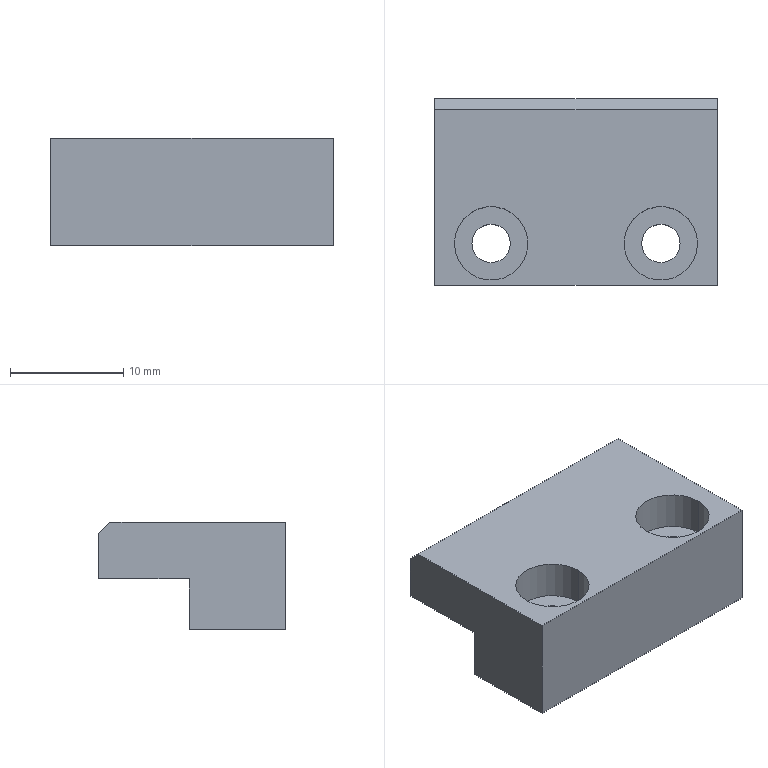Part | STEP file | PN_0054 | 1 solid | 19 faces | box 25 x 16.5 x 9.5 mm | volume 2670 mm3 | plane 11 | cylinder 8 | commonest cylinder face diameters 3.4 x4 6.5 x4
STEP:
#1=CARTESIAN_POINT('',(0.,0.,0.));
#2=DIRECTION('',(0.,0.,1.));
#3=DIRECTION('',(1.,0.,0.));
#4=AXIS2_PLACEMENT_3D('',#1,#2,#3);
#5=CARTESIAN_POINT('',(-4.25,-4.55,6.1));
#6=VERTEX_POINT('',#5);
#7=CARTESIAN_POINT('',(-4.25,-4.55,9.5));
#8=VERTEX_POINT('',#7);
#9=CARTESIAN_POINT('',(-4.25,-4.55,9.5));
#10=DIRECTION('',(0.,0.,1.));
#11=VECTOR('',#10,1.);
#12=LINE('',#9,#11);
#13=CARTESIAN_POINT('',(-7.5,-4.55,9.5));
#14=DIRECTION('',(0.,0.,1.));
#15=DIRECTION('',(1.,0.,0.));
#16=AXIS2_PLACEMENT_3D('',#13,#14,#15);
#17=CYLINDRICAL_SURFACE('',#16,3.25);
#18=CARTESIAN_POINT('',(6.283,0.));
#19=DIRECTION('',(0.,1.));
#20=VECTOR('',#19,1.);
#21=LINE('',#18,#20);
#22=(GEOMETRIC_REPRESENTATION_CONTEXT(2)PARAMETRIC_REPRESENTATION_CONTEXT()REPRESENTATION_CONTEXT('',''));
#23=DEFINITIONAL_REPRESENTATION('',(#21),#22);
#24=PCURVE('',#17,#23);
#25=CARTESIAN_POINT('',(-7.5,-4.55,9.5));
#26=DIRECTION('',(0.,0.,1.));
#27=DIRECTION('',(1.,0.,0.));
#28=AXIS2_PLACEMENT_3D('',#25,#26,#27);
#29=CYLINDRICAL_SURFACE('',#28,3.25);
#30=CARTESIAN_POINT('',(0.,0.));
#31=DIRECTION('',(0.,1.));
#32=VECTOR('',#31,1.);
#33=LINE('',#30,#32);
#34=(GEOMETRIC_REPRESENTATION_CONTEXT(2)PARAMETRIC_REPRESENTATION_CONTEXT()REPRESENTATION_CONTEXT('',''));
#35=DEFINITIONAL_REPRESENTATION('',(#33),#34);
#36=PCURVE('',#29,#35);
#37=SURFACE_CURVE('',#12,(#24,#36),.PCURVE_S1.);
#38=EDGE_CURVE('',#6,#8,#37,.T.);
#39=ORIENTED_EDGE('',*,*,#38,.T.);
#40=CARTESIAN_POINT('',(-10.75,-4.55,9.5));
#41=VERTEX_POINT('',#40);
#42=CARTESIAN_POINT('',(-7.5,-4.55,9.5));
#43=DIRECTION('',(0.,0.,1.));
#44=DIRECTION('',(1.,0.,0.));
#45=AXIS2_PLACEMENT_3D('',#42,#43,#44);
#46=CIRCLE('',#45,3.25);
#47=CARTESIAN_POINT('',(0.,0.));
#48=DIRECTION('',(1.,0.));
#49=VECTOR('',#48,1.);
#50=LINE('',#47,#49);
#51=(GEOMETRIC_REPRESENTATION_CONTEXT(2)PARAMETRIC_REPRESENTATION_CONTEXT()REPRESENTATION_CONTEXT('',''));
#52=DEFINITIONAL_REPRESENTATION('',(#50),#51);
#53=PCURVE('',#17,#52);
#54=CARTESIAN_POINT('',(0.,0.,9.5));
#55=DIRECTION('',(0.,0.,1.));
#56=DIRECTION('',(1.,0.,0.));
#57=AXIS2_PLACEMENT_3D('',#54,#55,#56);
#58=PLANE('',#57);
#59=CARTESIAN_POINT('',(-7.5,-4.55));
#60=DIRECTION('',(1.,0.));
#61=AXIS2_PLACEMENT_2D('',#59,#60);
#62=CIRCLE('',#61,3.25);
#63=(GEOMETRIC_REPRESENTATION_CONTEXT(2)PARAMETRIC_REPRESENTATION_CONTEXT()REPRESENTATION_CONTEXT('',''));
#64=DEFINITIONAL_REPRESENTATION('',(#62),#63);
#65=PCURVE('',#58,#64);
#66=SURFACE_CURVE('',#46,(#53,#65),.PCURVE_S1.);
#67=EDGE_CURVE('',#41,#8,#66,.T.);
#68=ORIENTED_EDGE('',*,*,#67,.F.);
#69=CARTESIAN_POINT('',(-10.75,-4.55,6.1));
#70=VERTEX_POINT('',#69);
#71=CARTESIAN_POINT('',(-10.75,-4.55,9.5));
#72=DIRECTION('',(0.,0.,1.));
#73=VECTOR('',#72,1.);
#74=LINE('',#71,#73);
#75=CARTESIAN_POINT('',(3.142,0.));
#76=DIRECTION('',(0.,1.));
#77=VECTOR('',#76,1.);
#78=LINE('',#75,#77);
#79=(GEOMETRIC_REPRESENTATION_CONTEXT(2)PARAMETRIC_REPRESENTATION_CONTEXT()REPRESENTATION_CONTEXT('',''));
#80=DEFINITIONAL_REPRESENTATION('',(#78),#79);
#81=PCURVE('',#17,#80);
#82=CARTESIAN_POINT('',(3.142,0.));
#83=DIRECTION('',(0.,1.));
#84=VECTOR('',#83,1.);
#85=LINE('',#82,#84);
#86=(GEOMETRIC_REPRESENTATION_CONTEXT(2)PARAMETRIC_REPRESENTATION_CONTEXT()REPRESENTATION_CONTEXT('',''));
#87=DEFINITIONAL_REPRESENTATION('',(#85),#86);
#88=PCURVE('',#29,#87);
#89=SURFACE_CURVE('',#74,(#81,#88),.PCURVE_S1.);
#90=EDGE_CURVE('',#70,#41,#89,.T.);
#91=ORIENTED_EDGE('',*,*,#90,.F.);
#92=CARTESIAN_POINT('',(-7.5,-4.55,6.1));
#93=DIRECTION('',(0.,0.,1.));
#94=DIRECTION('',(1.,0.,0.));
#95=AXIS2_PLACEMENT_3D('',#92,#93,#94);
#96=CIRCLE('',#95,3.25);
#97=CARTESIAN_POINT('',(0.,-3.4));
#98=DIRECTION('',(1.,0.));
#99=VECTOR('',#98,1.);
#100=LINE('',#97,#99);
#101=(GEOMETRIC_REPRESENTATION_CONTEXT(2)PARAMETRIC_REPRESENTATION_CONTEXT()REPRESENTATION_CONTEXT('',''));
#102=DEFINITIONAL_REPRESENTATION('',(#100),#101);
#103=PCURVE('',#17,#102);
#104=CARTESIAN_POINT('',(-5.8,-4.55,6.1));
#105=DIRECTION('',(0.,0.,-1.));
#106=DIRECTION('',(-1.,0.,0.));
#107=AXIS2_PLACEMENT_3D('',#104,#105,#106);
#108=PLANE('',#107);
#109=CARTESIAN_POINT('',(-1.55,0.));
#110=CARTESIAN_POINT('',(-1.55,5.629));
#111=CARTESIAN_POINT('',(3.325,2.815));
#112=CARTESIAN_POINT('',(8.2,0.));
#113=CARTESIAN_POINT('',(3.325,-2.815));
#114=CARTESIAN_POINT('',(-1.55,-5.629));
#115=CARTESIAN_POINT('',(-1.55,0.));
#116=(BOUNDED_CURVE()B_SPLINE_CURVE(2,(#109,#110,#111,#112,#113,#114,#115),.UNSPECIFIED.,.T.,.F.)B_SPLINE_CURVE_WITH_KNOTS((1,2,2,2,2,1),(-2.094,0.,2.094,4.189,6.283,8.378),.UNSPECIFIED.)CURVE()GEOMETRIC_REPRESENTATION_ITEM()RATIONAL_B_SPLINE_CURVE((1.,0.5,1.,0.5,1.,0.5,1.))REPRESENTATION_ITEM(''));
#117=(GEOMETRIC_REPRESENTATION_CONTEXT(2)PARAMETRIC_REPRESENTATION_CONTEXT()REPRESENTATION_CONTEXT('',''));
#118=DEFINITIONAL_REPRESENTATION('',(#116),#117);
#119=PCURVE('',#108,#118);
#120=SURFACE_CURVE('',#96,(#103,#119),.PCURVE_S1.);
#121=EDGE_CURVE('',#70,#6,#120,.T.);
#122=ORIENTED_EDGE('',*,*,#121,.T.);
#123=EDGE_LOOP('',(#39,#68,#91,#122));
#124=FACE_BOUND('',#123,.F.);
#125=ADVANCED_FACE('',(#124),#17,.F.);
#126=CARTESIAN_POINT('',(-5.8,-4.55,0.));
#127=VERTEX_POINT('',#126);
#128=CARTESIAN_POINT('',(-5.8,-4.55,6.1));
#129=VERTEX_POINT('',#128);
#130=CARTESIAN_POINT('',(-5.8,-4.55,9.5));
#131=DIRECTION('',(0.,0.,1.));
#132=VECTOR('',#131,1.);
#133=LINE('',#130,#132);
#134=CARTESIAN_POINT('',(-7.5,-4.55,9.5));
#135=DIRECTION('',(0.,0.,1.));
#136=DIRECTION('',(1.,0.,0.));
#137=AXIS2_PLACEMENT_3D('',#134,#135,#136);
#138=CYLINDRICAL_SURFACE('',#137,1.7);
#139=CARTESIAN_POINT('',(6.283,0.));
#140=DIRECTION('',(0.,1.));
#141=VECTOR('',#140,1.);
#142=LINE('',#139,#141);
#143=(GEOMETRIC_REPRESENTATION_CONTEXT(2)PARAMETRIC_REPRESENTATION_CONTEXT()REPRESENTATION_CONTEXT('',''));
#144=DEFINITIONAL_REPRESENTATION('',(#142),#143);
#145=PCURVE('',#138,#144);
#146=CARTESIAN_POINT('',(-7.5,-4.55,9.5));
#147=DIRECTION('',(0.,0.,1.));
#148=DIRECTION('',(1.,0.,0.));
#149=AXIS2_PLACEMENT_3D('',#146,#147,#148);
#150=CYLINDRICAL_SURFACE('',#149,1.7);
#151=CARTESIAN_POINT('',(0.,0.));
#152=DIRECTION('',(0.,1.));
#153=VECTOR('',#152,1.);
#154=LINE('',#151,#153);
#155=(GEOMETRIC_REPRESENTATION_CONTEXT(2)PARAMETRIC_REPRESENTATION_CONTEXT()REPRESENTATION_CONTEXT('',''));
#156=DEFINITIONAL_REPRESENTATION('',(#154),#155);
#157=PCURVE('',#150,#156);
#158=SURFACE_CURVE('',#133,(#145,#157),.PCURVE_S1.);
#159=EDGE_CURVE('',#127,#129,#158,.T.);
#160=ORIENTED_EDGE('',*,*,#159,.T.);
#161=CARTESIAN_POINT('',(-9.2,-4.55,6.1));
#162=VERTEX_POINT('',#161);
#163=CARTESIAN_POINT('',(-7.5,-4.55,6.1));
#164=DIRECTION('',(0.,0.,1.));
#165=DIRECTION('',(1.,0.,0.));
#166=AXIS2_PLACEMENT_3D('',#163,#164,#165);
#167=CIRCLE('',#166,1.7);
#168=CARTESIAN_POINT('',(0.,-3.4));
#169=DIRECTION('',(1.,0.));
#170=VECTOR('',#169,1.);
#171=LINE('',#168,#170);
#172=(GEOMETRIC_REPRESENTATION_CONTEXT(2)PARAMETRIC_REPRESENTATION_CONTEXT()REPRESENTATION_CONTEXT('',''));
#173=DEFINITIONAL_REPRESENTATION('',(#171),#172);
#174=PCURVE('',#138,#173);
#175=CARTESIAN_POINT('',(0.,0.));
#176=CARTESIAN_POINT('',(0.,2.944));
#177=CARTESIAN_POINT('',(2.55,1.472));
#178=CARTESIAN_POINT('',(5.1,0.));
#179=CARTESIAN_POINT('',(2.55,-1.472));
#180=CARTESIAN_POINT('',(0.,-2.944));
#181=CARTESIAN_POINT('',(0.,0.));
#182=(BOUNDED_CURVE()B_SPLINE_CURVE(2,(#175,#176,#177,#178,#179,#180,#181),.UNSPECIFIED.,.T.,.F.)B_SPLINE_CURVE_WITH_KNOTS((1,2,2,2,2,1),(-2.094,0.,2.094,4.189,6.283,8.378),.UNSPECIFIED.)CURVE()GEOMETRIC_REPRESENTATION_ITEM()RATIONAL_B_SPLINE_CURVE((1.,0.5,1.,0.5,1.,0.5,1.))REPRESENTATION_ITEM(''));
#183=(GEOMETRIC_REPRESENTATION_CONTEXT(2)PARAMETRIC_REPRESENTATION_CONTEXT()REPRESENTATION_CONTEXT('',''));
#184=DEFINITIONAL_REPRESENTATION('',(#182),#183);
#185=PCURVE('',#108,#184);
#186=SURFACE_CURVE('',#167,(#174,#185),.PCURVE_S1.);
#187=EDGE_CURVE('',#162,#129,#186,.T.);
#188=ORIENTED_EDGE('',*,*,#187,.F.);
#189=CARTESIAN_POINT('',(-9.2,-4.55,0.));
#190=VERTEX_POINT('',#189);
#191=CARTESIAN_POINT('',(-9.2,-4.55,9.5));
#192=DIRECTION('',(0.,0.,1.));
#193=VECTOR('',#192,1.);
#194=LINE('',#191,#193);
#195=CARTESIAN_POINT('',(3.142,0.));
#196=DIRECTION('',(0.,1.));
#197=VECTOR('',#196,1.);
#198=LINE('',#195,#197);
#199=(GEOMETRIC_REPRESENTATION_CONTEXT(2)PARAMETRIC_REPRESENTATION_CONTEXT()REPRESENTATION_CONTEXT('',''));
#200=DEFINITIONAL_REPRESENTATION('',(#198),#199);
#201=PCURVE('',#138,#200);
#202=CARTESIAN_POINT('',(3.142,0.));
#203=DIRECTION('',(0.,1.));
#204=VECTOR('',#203,1.);
#205=LINE('',#202,#204);
#206=(GEOMETRIC_REPRESENTATION_CONTEXT(2)PARAMETRIC_REPRESENTATION_CONTEXT()REPRESENTATION_CONTEXT('',''));
#207=DEFINITIONAL_REPRESENTATION('',(#205),#206);
#208=PCURVE('',#150,#207);
#209=SURFACE_CURVE('',#194,(#201,#208),.PCURVE_S1.);
#210=EDGE_CURVE('',#190,#162,#209,.T.);
#211=ORIENTED_EDGE('',*,*,#210,.F.);
#212=CARTESIAN_POINT('',(-7.5,-4.55,0.));
#213=DIRECTION('',(0.,0.,1.));
#214=DIRECTION('',(1.,0.,0.));
#215=AXIS2_PLACEMENT_3D('',#212,#213,#214);
#216=CIRCLE('',#215,1.7);
#217=CARTESIAN_POINT('',(0.,-9.5));
#218=DIRECTION('',(1.,0.));
#219=VECTOR('',#218,1.);
#220=LINE('',#217,#219);
#221=(GEOMETRIC_REPRESENTATION_CONTEXT(2)PARAMETRIC_REPRESENTATION_CONTEXT()REPRESENTATION_CONTEXT('',''));
#222=DEFINITIONAL_REPRESENTATION('',(#220),#221);
#223=PCURVE('',#138,#222);
#224=CARTESIAN_POINT('',(0.,0.,0.));
#225=DIRECTION('',(0.,0.,1.));
#226=DIRECTION('',(1.,0.,0.));
#227=AXIS2_PLACEMENT_3D('',#224,#225,#226);
#228=PLANE('',#227);
#229=CARTESIAN_POINT('',(-7.5,-4.55));
#230=DIRECTION('',(1.,0.));
#231=AXIS2_PLACEMENT_2D('',#229,#230);
#232=CIRCLE('',#231,1.7);
#233=(GEOMETRIC_REPRESENTATION_CONTEXT(2)PARAMETRIC_REPRESENTATION_CONTEXT()REPRESENTATION_CONTEXT('',''));
#234=DEFINITIONAL_REPRESENTATION('',(#232),#233);
#235=PCURVE('',#228,#234);
#236=SURFACE_CURVE('',#216,(#223,#235),.PCURVE_S1.);
#237=EDGE_CURVE('',#190,#127,#236,.T.);
#238=ORIENTED_EDGE('',*,*,#237,.T.);
#239=EDGE_LOOP('',(#160,#188,#211,#238));
#240=FACE_BOUND('',#239,.F.);
#241=ADVANCED_FACE('',(#240),#138,.F.);
#242=CARTESIAN_POINT('',(10.75,-4.55,6.1));
#243=VERTEX_POINT('',#242);
#244=CARTESIAN_POINT('',(10.75,-4.55,9.5));
#245=VERTEX_POINT('',#244);
#246=CARTESIAN_POINT('',(10.75,-4.55,9.5));
#247=DIRECTION('',(0.,0.,1.));
#248=VECTOR('',#247,1.);
#249=LINE('',#246,#248);
#250=CARTESIAN_POINT('',(7.5,-4.55,9.5));
#251=DIRECTION('',(0.,0.,1.));
#252=DIRECTION('',(1.,0.,0.));
#253=AXIS2_PLACEMENT_3D('',#250,#251,#252);
#254=CYLINDRICAL_SURFACE('',#253,3.25);
#255=CARTESIAN_POINT('',(6.283,0.));
#256=DIRECTION('',(0.,1.));
#257=VECTOR('',#256,1.);
#258=LINE('',#255,#257);
#259=(GEOMETRIC_REPRESENTATION_CONTEXT(2)PARAMETRIC_REPRESENTATION_CONTEXT()REPRESENTATION_CONTEXT('',''));
#260=DEFINITIONAL_REPRESENTATION('',(#258),#259);
#261=PCURVE('',#254,#260);
#262=CARTESIAN_POINT('',(7.5,-4.55,9.5));
#263=DIRECTION('',(0.,0.,1.));
#264=DIRECTION('',(1.,0.,0.));
#265=AXIS2_PLACEMENT_3D('',#262,#263,#264);
#266=CYLINDRICAL_SURFACE('',#265,3.25);
#267=CARTESIAN_POINT('',(0.,0.));
#268=DIRECTION('',(0.,1.));
#269=VECTOR('',#268,1.);
#270=LINE('',#267,#269);
#271=(GEOMETRIC_REPRESENTATION_CONTEXT(2)PARAMETRIC_REPRESENTATION_CONTEXT()REPRESENTATION_CONTEXT('',''));
#272=DEFINITIONAL_REPRESENTATION('',(#270),#271);
#273=PCURVE('',#266,#272);
#274=SURFACE_CURVE('',#249,(#261,#273),.PCURVE_S1.);
#275=EDGE_CURVE('',#243,#245,#274,.T.);
#276=ORIENTED_EDGE('',*,*,#275,.T.);
#277=CARTESIAN_POINT('',(4.25,-4.55,9.5));
#278=VERTEX_POINT('',#277);
#279=CARTESIAN_POINT('',(7.5,-4.55,9.5));
#280=DIRECTION('',(0.,0.,1.));
#281=DIRECTION('',(1.,0.,0.));
#282=AXIS2_PLACEMENT_3D('',#279,#280,#281);
#283=CIRCLE('',#282,3.25);
#284=CARTESIAN_POINT('',(0.,0.));
#285=DIRECTION('',(1.,0.));
#286=VECTOR('',#285,1.);
#287=LINE('',#284,#286);
#288=(GEOMETRIC_REPRESENTATION_CONTEXT(2)PARAMETRIC_REPRESENTATION_CONTEXT()REPRESENTATION_CONTEXT('',''));
#289=DEFINITIONAL_REPRESENTATION('',(#287),#288);
#290=PCURVE('',#254,#289);
#291=CARTESIAN_POINT('',(7.5,-4.55));
#292=DIRECTION('',(1.,0.));
#293=AXIS2_PLACEMENT_2D('',#291,#292);
#294=CIRCLE('',#293,3.25);
#295=(GEOMETRIC_REPRESENTATION_CONTEXT(2)PARAMETRIC_REPRESENTATION_CONTEXT()REPRESENTATION_CONTEXT('',''));
#296=DEFINITIONAL_REPRESENTATION('',(#294),#295);
#297=PCURVE('',#58,#296);
#298=SURFACE_CURVE('',#283,(#290,#297),.PCURVE_S1.);
#299=EDGE_CURVE('',#278,#245,#298,.T.);
#300=ORIENTED_EDGE('',*,*,#299,.F.);
#301=CARTESIAN_POINT('',(4.25,-4.55,6.1));
#302=VERTEX_POINT('',#301);
#303=CARTESIAN_POINT('',(4.25,-4.55,9.5));
#304=DIRECTION('',(0.,0.,1.));
#305=VECTOR('',#304,1.);
#306=LINE('',#303,#305);
#307=CARTESIAN_POINT('',(3.142,0.));
#308=DIRECTION('',(0.,1.));
#309=VECTOR('',#308,1.);
#310=LINE('',#307,#309);
#311=(GEOMETRIC_REPRESENTATION_CONTEXT(2)PARAMETRIC_REPRESENTATION_CONTEXT()REPRESENTATION_CONTEXT('',''));
#312=DEFINITIONAL_REPRESENTATION('',(#310),#311);
#313=PCURVE('',#254,#312);
#314=CARTESIAN_POINT('',(3.142,0.));
#315=DIRECTION('',(0.,1.));
#316=VECTOR('',#315,1.);
#317=LINE('',#314,#316);
#318=(GEOMETRIC_REPRESENTATION_CONTEXT(2)PARAMETRIC_REPRESENTATION_CONTEXT()REPRESENTATION_CONTEXT('',''));
#319=DEFINITIONAL_REPRESENTATION('',(#317),#318);
#320=PCURVE('',#266,#319);
#321=SURFACE_CURVE('',#306,(#313,#320),.PCURVE_S1.);
#322=EDGE_CURVE('',#302,#278,#321,.T.);
#323=ORIENTED_EDGE('',*,*,#322,.F.);
#324=CARTESIAN_POINT('',(7.5,-4.55,6.1));
#325=DIRECTION('',(0.,0.,1.));
#326=DIRECTION('',(1.,0.,0.));
#327=AXIS2_PLACEMENT_3D('',#324,#325,#326);
#328=CIRCLE('',#327,3.25);
#329=CARTESIAN_POINT('',(0.,-3.4));
#330=DIRECTION('',(1.,0.));
#331=VECTOR('',#330,1.);
#332=LINE('',#329,#331);
#333=(GEOMETRIC_REPRESENTATION_CONTEXT(2)PARAMETRIC_REPRESENTATION_CONTEXT()REPRESENTATION_CONTEXT('',''));
#334=DEFINITIONAL_REPRESENTATION('',(#332),#333);
#335=PCURVE('',#254,#334);
#336=CARTESIAN_POINT('',(9.2,-4.55,6.1));
#337=DIRECTION('',(0.,0.,-1.));
#338=DIRECTION('',(-1.,0.,0.));
#339=AXIS2_PLACEMENT_3D('',#336,#337,#338);
#340=PLANE('',#339);
#341=CARTESIAN_POINT('',(-1.55,0.));
#342=CARTESIAN_POINT('',(-1.55,5.629));
#343=CARTESIAN_POINT('',(3.325,2.815));
#344=CARTESIAN_POINT('',(8.2,0.));
#345=CARTESIAN_POINT('',(3.325,-2.815));
#346=CARTESIAN_POINT('',(-1.55,-5.629));
#347=CARTESIAN_POINT('',(-1.55,0.));
#348=(BOUNDED_CURVE()B_SPLINE_CURVE(2,(#341,#342,#343,#344,#345,#346,#347),.UNSPECIFIED.,.T.,.F.)B_SPLINE_CURVE_WITH_KNOTS((1,2,2,2,2,1),(-2.094,0.,2.094,4.189,6.283,8.378),.UNSPECIFIED.)CURVE()GEOMETRIC_REPRESENTATION_ITEM()RATIONAL_B_SPLINE_CURVE((1.,0.5,1.,0.5,1.,0.5,1.))REPRESENTATION_ITEM(''));
#349=(GEOMETRIC_REPRESENTATION_CONTEXT(2)PARAMETRIC_REPRESENTATION_CONTEXT()REPRESENTATION_CONTEXT('',''));
#350=DEFINITIONAL_REPRESENTATION('',(#348),#349);
#351=PCURVE('',#340,#350);
#352=SURFACE_CURVE('',#328,(#335,#351),.PCURVE_S1.);
#353=EDGE_CURVE('',#302,#243,#352,.T.);
#354=ORIENTED_EDGE('',*,*,#353,.T.);
#355=EDGE_LOOP('',(#276,#300,#323,#354));
#356=FACE_BOUND('',#355,.F.);
#357=ADVANCED_FACE('',(#356),#254,.F.);
#358=CARTESIAN_POINT('',(9.2,-4.55,0.));
#359=VERTEX_POINT('',#358);
#360=CARTESIAN_POINT('',(9.2,-4.55,6.1));
#361=VERTEX_POINT('',#360);
#362=CARTESIAN_POINT('',(9.2,-4.55,9.5));
#363=DIRECTION('',(0.,0.,1.));
#364=VECTOR('',#363,1.);
#365=LINE('',#362,#364);
#366=CARTESIAN_POINT('',(7.5,-4.55,9.5));
#367=DIRECTION('',(0.,0.,1.));
#368=DIRECTION('',(1.,0.,0.));
#369=AXIS2_PLACEMENT_3D('',#366,#367,#368);
#370=CYLINDRICAL_SURFACE('',#369,1.7);
#371=CARTESIAN_POINT('',(6.283,0.));
#372=DIRECTION('',(0.,1.));
#373=VECTOR('',#372,1.);
#374=LINE('',#371,#373);
#375=(GEOMETRIC_REPRESENTATION_CONTEXT(2)PARAMETRIC_REPRESENTATION_CONTEXT()REPRESENTATION_CONTEXT('',''));
#376=DEFINITIONAL_REPRESENTATION('',(#374),#375);
#377=PCURVE('',#370,#376);
#378=CARTESIAN_POINT('',(7.5,-4.55,9.5));
#379=DIRECTION('',(0.,0.,1.));
#380=DIRECTION('',(1.,0.,0.));
#381=AXIS2_PLACEMENT_3D('',#378,#379,#380);
#382=CYLINDRICAL_SURFACE('',#381,1.7);
#383=CARTESIAN_POINT('',(0.,0.));
#384=DIRECTION('',(0.,1.));
#385=VECTOR('',#384,1.);
#386=LINE('',#383,#385);
#387=(GEOMETRIC_REPRESENTATION_CONTEXT(2)PARAMETRIC_REPRESENTATION_CONTEXT()REPRESENTATION_CONTEXT('',''));
#388=DEFINITIONAL_REPRESENTATION('',(#386),#387);
#389=PCURVE('',#382,#388);
#390=SURFACE_CURVE('',#365,(#377,#389),.PCURVE_S1.);
#391=EDGE_CURVE('',#359,#361,#390,.T.);
#392=ORIENTED_EDGE('',*,*,#391,.T.);
#393=CARTESIAN_POINT('',(5.8,-4.55,6.1));
#394=VERTEX_POINT('',#393);
#395=CARTESIAN_POINT('',(7.5,-4.55,6.1));
#396=DIRECTION('',(0.,0.,1.));
#397=DIRECTION('',(1.,0.,0.));
#398=AXIS2_PLACEMENT_3D('',#395,#396,#397);
#399=CIRCLE('',#398,1.7);
#400=CARTESIAN_POINT('',(0.,-3.4));
#401=DIRECTION('',(1.,0.));
#402=VECTOR('',#401,1.);
#403=LINE('',#400,#402);
#404=(GEOMETRIC_REPRESENTATION_CONTEXT(2)PARAMETRIC_REPRESENTATION_CONTEXT()REPRESENTATION_CONTEXT('',''));
#405=DEFINITIONAL_REPRESENTATION('',(#403),#404);
#406=PCURVE('',#370,#405);
#407=CARTESIAN_POINT('',(0.,0.));
#408=CARTESIAN_POINT('',(0.,2.944));
#409=CARTESIAN_POINT('',(2.55,1.472));
#410=CARTESIAN_POINT('',(5.1,0.));
#411=CARTESIAN_POINT('',(2.55,-1.472));
#412=CARTESIAN_POINT('',(0.,-2.944));
#413=CARTESIAN_POINT('',(0.,0.));
#414=(BOUNDED_CURVE()B_SPLINE_CURVE(2,(#407,#408,#409,#410,#411,#412,#413),.UNSPECIFIED.,.T.,.F.)B_SPLINE_CURVE_WITH_KNOTS((1,2,2,2,2,1),(-2.094,0.,2.094,4.189,6.283,8.378),.UNSPECIFIED.)CURVE()GEOMETRIC_REPRESENTATION_ITEM()RATIONAL_B_SPLINE_CURVE((1.,0.5,1.,0.5,1.,0.5,1.))REPRESENTATION_ITEM(''));
#415=(GEOMETRIC_REPRESENTATION_CONTEXT(2)PARAMETRIC_REPRESENTATION_CONTEXT()REPRESENTATION_CONTEXT('',''));
#416=DEFINITIONAL_REPRESENTATION('',(#414),#415);
#417=PCURVE('',#340,#416);
#418=SURFACE_CURVE('',#399,(#406,#417),.PCURVE_S1.);
#419=EDGE_CURVE('',#394,#361,#418,.T.);
#420=ORIENTED_EDGE('',*,*,#419,.F.);
#421=CARTESIAN_POINT('',(5.8,-4.55,0.));
#422=VERTEX_POINT('',#421);
#423=CARTESIAN_POINT('',(5.8,-4.55,9.5));
#424=DIRECTION('',(0.,0.,1.));
#425=VECTOR('',#424,1.);
#426=LINE('',#423,#425);
#427=CARTESIAN_POINT('',(3.142,0.));
#428=DIRECTION('',(0.,1.));
#429=VECTOR('',#428,1.);
#430=LINE('',#427,#429);
#431=(GEOMETRIC_REPRESENTATION_CONTEXT(2)PARAMETRIC_REPRESENTATION_CONTEXT()REPRESENTATION_CONTEXT('',''));
#432=DEFINITIONAL_REPRESENTATION('',(#430),#431);
#433=PCURVE('',#370,#432);
#434=CARTESIAN_POINT('',(3.142,0.));
#435=DIRECTION('',(0.,1.));
#436=VECTOR('',#435,1.);
#437=LINE('',#434,#436);
#438=(GEOMETRIC_REPRESENTATION_CONTEXT(2)PARAMETRIC_REPRESENTATION_CONTEXT()REPRESENTATION_CONTEXT('',''));
#439=DEFINITIONAL_REPRESENTATION('',(#437),#438);
#440=PCURVE('',#382,#439);
#441=SURFACE_CURVE('',#426,(#433,#440),.PCURVE_S1.);
#442=EDGE_CURVE('',#422,#394,#441,.T.);
#443=ORIENTED_EDGE('',*,*,#442,.F.);
#444=CARTESIAN_POINT('',(7.5,-4.55,0.));
#445=DIRECTION('',(0.,0.,1.));
#446=DIRECTION('',(1.,0.,0.));
#447=AXIS2_PLACEMENT_3D('',#444,#445,#446);
#448=CIRCLE('',#447,1.7);
#449=CARTESIAN_POINT('',(0.,-9.5));
#450=DIRECTION('',(1.,0.));
#451=VECTOR('',#450,1.);
#452=LINE('',#449,#451);
#453=(GEOMETRIC_REPRESENTATION_CONTEXT(2)PARAMETRIC_REPRESENTATION_CONTEXT()REPRESENTATION_CONTEXT('',''));
#454=DEFINITIONAL_REPRESENTATION('',(#452),#453);
#455=PCURVE('',#370,#454);
#456=CARTESIAN_POINT('',(7.5,-4.55));
#457=DIRECTION('',(1.,0.));
#458=AXIS2_PLACEMENT_2D('',#456,#457);
#459=CIRCLE('',#458,1.7);
#460=(GEOMETRIC_REPRESENTATION_CONTEXT(2)PARAMETRIC_REPRESENTATION_CONTEXT()REPRESENTATION_CONTEXT('',''));
#461=DEFINITIONAL_REPRESENTATION('',(#459),#460);
#462=PCURVE('',#228,#461);
#463=SURFACE_CURVE('',#448,(#455,#462),.PCURVE_S1.);
#464=EDGE_CURVE('',#422,#359,#463,.T.);
#465=ORIENTED_EDGE('',*,*,#464,.T.);
#466=EDGE_LOOP('',(#392,#420,#443,#465));
#467=FACE_BOUND('',#466,.F.);
#468=ADVANCED_FACE('',(#467),#370,.F.);
#469=CARTESIAN_POINT('',(12.5,8.25,8.5));
#470=VERTEX_POINT('',#469);
#471=CARTESIAN_POINT('',(12.5,8.25,4.5));
#472=VERTEX_POINT('',#471);
#473=CARTESIAN_POINT('',(12.5,8.25,9.5));
#474=DIRECTION('',(0.,0.,-1.));
#475=VECTOR('',#474,1.);
#476=LINE('',#473,#475);
#477=CARTESIAN_POINT('',(12.5,8.25,9.5));
#478=DIRECTION('',(-1.,0.,0.));
#479=DIRECTION('',(0.,-1.,0.));
#480=AXIS2_PLACEMENT_3D('',#477,#478,#479);
#481=PLANE('',#480);
#482=CARTESIAN_POINT('',(0.,0.));
#483=DIRECTION('',(0.,-1.));
#484=VECTOR('',#483,1.);
#485=LINE('',#482,#484);
#486=(GEOMETRIC_REPRESENTATION_CONTEXT(2)PARAMETRIC_REPRESENTATION_CONTEXT()REPRESENTATION_CONTEXT('',''));
#487=DEFINITIONAL_REPRESENTATION('',(#485),#486);
#488=PCURVE('',#481,#487);
#489=CARTESIAN_POINT('',(-12.5,8.25,9.5));
#490=DIRECTION('',(0.,-1.,0.));
#491=DIRECTION('',(0.,0.,-1.));
#492=AXIS2_PLACEMENT_3D('',#489,#490,#491);
#493=PLANE('',#492);
#494=CARTESIAN_POINT('',(0.,25.));
#495=DIRECTION('',(1.,0.));
#496=VECTOR('',#495,1.);
#497=LINE('',#494,#496);
#498=(GEOMETRIC_REPRESENTATION_CONTEXT(2)PARAMETRIC_REPRESENTATION_CONTEXT()REPRESENTATION_CONTEXT('',''));
#499=DEFINITIONAL_REPRESENTATION('',(#497),#498);
#500=PCURVE('',#493,#499);
#501=SURFACE_CURVE('',#476,(#488,#500),.PCURVE_S1.);
#502=EDGE_CURVE('',#470,#472,#501,.T.);
#503=ORIENTED_EDGE('',*,*,#502,.F.);
#504=CARTESIAN_POINT('',(12.5,7.25,9.5));
#505=VERTEX_POINT('',#504);
#506=CARTESIAN_POINT('',(12.5,7.25,9.5));
#507=DIRECTION('',(0.,-0.7071,0.7071));
#508=VECTOR('',#507,1.);
#509=LINE('',#506,#508);
#510=CARTESIAN_POINT('',(1.,0.));
#511=DIRECTION('',(0.7071,0.7071));
#512=VECTOR('',#511,1.);
#513=LINE('',#510,#512);
#514=(GEOMETRIC_REPRESENTATION_CONTEXT(2)PARAMETRIC_REPRESENTATION_CONTEXT()REPRESENTATION_CONTEXT('',''));
#515=DEFINITIONAL_REPRESENTATION('',(#513),#514);
#516=PCURVE('',#481,#515);
#517=CARTESIAN_POINT('',(0.,7.25,9.5));
#518=DIRECTION('',(0.,0.7071,0.7071));
#519=DIRECTION('',(1.,0.,0.));
#520=AXIS2_PLACEMENT_3D('',#517,#518,#519);
#521=PLANE('',#520);
#522=CARTESIAN_POINT('',(12.5,0.));
#523=DIRECTION('',(0.,-1.));
#524=VECTOR('',#523,1.);
#525=LINE('',#522,#524);
#526=(GEOMETRIC_REPRESENTATION_CONTEXT(2)PARAMETRIC_REPRESENTATION_CONTEXT()REPRESENTATION_CONTEXT('',''));
#527=DEFINITIONAL_REPRESENTATION('',(#525),#526);
#528=PCURVE('',#521,#527);
#529=SURFACE_CURVE('',#509,(#516,#528),.PCURVE_S1.);
#530=EDGE_CURVE('',#470,#505,#529,.T.);
#531=ORIENTED_EDGE('',*,*,#530,.T.);
#532=CARTESIAN_POINT('',(12.5,-8.25,9.5));
#533=VERTEX_POINT('',#532);
#534=CARTESIAN_POINT('',(12.5,8.25,9.5));
#535=DIRECTION('',(0.,1.,0.));
#536=VECTOR('',#535,1.);
#537=LINE('',#534,#536);
#538=CARTESIAN_POINT('',(0.,0.));
#539=DIRECTION('',(-1.,0.));
#540=VECTOR('',#539,1.);
#541=LINE('',#538,#540);
#542=(GEOMETRIC_REPRESENTATION_CONTEXT(2)PARAMETRIC_REPRESENTATION_CONTEXT()REPRESENTATION_CONTEXT('',''));
#543=DEFINITIONAL_REPRESENTATION('',(#541),#542);
#544=PCURVE('',#481,#543);
#545=CARTESIAN_POINT('',(12.5,8.25));
#546=DIRECTION('',(0.,1.));
#547=VECTOR('',#546,1.);
#548=LINE('',#545,#547);
#549=(GEOMETRIC_REPRESENTATION_CONTEXT(2)PARAMETRIC_REPRESENTATION_CONTEXT()REPRESENTATION_CONTEXT('',''));
#550=DEFINITIONAL_REPRESENTATION('',(#548),#549);
#551=PCURVE('',#58,#550);
#552=SURFACE_CURVE('',#537,(#544,#551),.PCURVE_S1.);
#553=EDGE_CURVE('',#533,#505,#552,.T.);
#554=ORIENTED_EDGE('',*,*,#553,.F.);
#555=CARTESIAN_POINT('',(12.5,-8.25,0.));
#556=VERTEX_POINT('',#555);
#557=CARTESIAN_POINT('',(12.5,-8.25,9.5));
#558=DIRECTION('',(0.,0.,-1.));
#559=VECTOR('',#558,1.);
#560=LINE('',#557,#559);
#561=CARTESIAN_POINT('',(16.5,0.));
#562=DIRECTION('',(0.,-1.));
#563=VECTOR('',#562,1.);
#564=LINE('',#561,#563);
#565=(GEOMETRIC_REPRESENTATION_CONTEXT(2)PARAMETRIC_REPRESENTATION_CONTEXT()REPRESENTATION_CONTEXT('',''));
#566=DEFINITIONAL_REPRESENTATION('',(#564),#565);
#567=PCURVE('',#481,#566);
#568=CARTESIAN_POINT('',(-12.5,-8.25,9.5));
#569=DIRECTION('',(0.,1.,0.));
#570=DIRECTION('',(0.,0.,1.));
#571=AXIS2_PLACEMENT_3D('',#568,#569,#570);
#572=PLANE('',#571);
#573=CARTESIAN_POINT('',(0.,25.));
#574=DIRECTION('',(-1.,0.));
#575=VECTOR('',#574,1.);
#576=LINE('',#573,#575);
#577=(GEOMETRIC_REPRESENTATION_CONTEXT(2)PARAMETRIC_REPRESENTATION_CONTEXT()REPRESENTATION_CONTEXT('',''));
#578=DEFINITIONAL_REPRESENTATION('',(#576),#577);
#579=PCURVE('',#572,#578);
#580=SURFACE_CURVE('',#560,(#567,#579),.PCURVE_S1.);
#581=EDGE_CURVE('',#533,#556,#580,.T.);
#582=ORIENTED_EDGE('',*,*,#581,.T.);
#583=CARTESIAN_POINT('',(12.5,0.25,0.));
#584=VERTEX_POINT('',#583);
#585=CARTESIAN_POINT('',(12.5,8.25,0.));
#586=DIRECTION('',(0.,1.,0.));
#587=VECTOR('',#586,1.);
#588=LINE('',#585,#587);
#589=CARTESIAN_POINT('',(0.,-9.5));
#590=DIRECTION('',(-1.,0.));
#591=VECTOR('',#590,1.);
#592=LINE('',#589,#591);
#593=(GEOMETRIC_REPRESENTATION_CONTEXT(2)PARAMETRIC_REPRESENTATION_CONTEXT()REPRESENTATION_CONTEXT('',''));
#594=DEFINITIONAL_REPRESENTATION('',(#592),#593);
#595=PCURVE('',#481,#594);
#596=CARTESIAN_POINT('',(12.5,8.25));
#597=DIRECTION('',(0.,1.));
#598=VECTOR('',#597,1.);
#599=LINE('',#596,#598);
#600=(GEOMETRIC_REPRESENTATION_CONTEXT(2)PARAMETRIC_REPRESENTATION_CONTEXT()REPRESENTATION_CONTEXT('',''));
#601=DEFINITIONAL_REPRESENTATION('',(#599),#600);
#602=PCURVE('',#228,#601);
#603=SURFACE_CURVE('',#588,(#595,#602),.PCURVE_S1.);
#604=EDGE_CURVE('',#556,#584,#603,.T.);
#605=ORIENTED_EDGE('',*,*,#604,.T.);
#606=CARTESIAN_POINT('',(12.5,0.25,4.5));
#607=VERTEX_POINT('',#606);
#608=CARTESIAN_POINT('',(12.5,0.25,4.5));
#609=DIRECTION('',(0.,0.,-1.));
#610=VECTOR('',#609,1.);
#611=LINE('',#608,#610);
#612=CARTESIAN_POINT('',(8.,-5.));
#613=DIRECTION('',(0.,-1.));
#614=VECTOR('',#613,1.);
#615=LINE('',#612,#614);
#616=(GEOMETRIC_REPRESENTATION_CONTEXT(2)PARAMETRIC_REPRESENTATION_CONTEXT()REPRESENTATION_CONTEXT('',''));
#617=DEFINITIONAL_REPRESENTATION('',(#615),#616);
#618=PCURVE('',#481,#617);
#619=CARTESIAN_POINT('',(-12.5,0.25,4.5));
#620=DIRECTION('',(0.,-1.,0.));
#621=DIRECTION('',(1.,0.,0.));
#622=AXIS2_PLACEMENT_3D('',#619,#620,#621);
#623=PLANE('',#622);
#624=CARTESIAN_POINT('',(25.,0.));
#625=DIRECTION('',(0.,-1.));
#626=VECTOR('',#625,1.);
#627=LINE('',#624,#626);
#628=(GEOMETRIC_REPRESENTATION_CONTEXT(2)PARAMETRIC_REPRESENTATION_CONTEXT()REPRESENTATION_CONTEXT('',''));
#629=DEFINITIONAL_REPRESENTATION('',(#627),#628);
#630=PCURVE('',#623,#629);
#631=SURFACE_CURVE('',#611,(#618,#630),.PCURVE_S1.);
#632=EDGE_CURVE('',#607,#584,#631,.T.);
#633=ORIENTED_EDGE('',*,*,#632,.F.);
#634=CARTESIAN_POINT('',(12.5,8.25,4.5));
#635=DIRECTION('',(0.,-1.,0.));
#636=VECTOR('',#635,1.);
#637=LINE('',#634,#636);
#638=CARTESIAN_POINT('',(0.,-5.));
#639=DIRECTION('',(1.,0.));
#640=VECTOR('',#639,1.);
#641=LINE('',#638,#640);
#642=(GEOMETRIC_REPRESENTATION_CONTEXT(2)PARAMETRIC_REPRESENTATION_CONTEXT()REPRESENTATION_CONTEXT('',''));
#643=DEFINITIONAL_REPRESENTATION('',(#641),#642);
#644=PCURVE('',#481,#643);
#645=CARTESIAN_POINT('',(-12.5,8.25,4.5));
#646=DIRECTION('',(0.,0.,1.));
#647=DIRECTION('',(1.,0.,0.));
#648=AXIS2_PLACEMENT_3D('',#645,#646,#647);
#649=PLANE('',#648);
#650=CARTESIAN_POINT('',(25.,0.));
#651=DIRECTION('',(0.,-1.));
#652=VECTOR('',#651,1.);
#653=LINE('',#650,#652);
#654=(GEOMETRIC_REPRESENTATION_CONTEXT(2)PARAMETRIC_REPRESENTATION_CONTEXT()REPRESENTATION_CONTEXT('',''));
#655=DEFINITIONAL_REPRESENTATION('',(#653),#654);
#656=PCURVE('',#649,#655);
#657=SURFACE_CURVE('',#637,(#644,#656),.PCURVE_S1.);
#658=EDGE_CURVE('',#472,#607,#657,.T.);
#659=ORIENTED_EDGE('',*,*,#658,.F.);
#660=EDGE_LOOP('',(#503,#531,#554,#582,#605,#633,#659));
#661=FACE_BOUND('',#660,.T.);
#662=ADVANCED_FACE('',(#661),#481,.F.);
#663=CARTESIAN_POINT('',(-12.5,8.25,8.5));
#664=VERTEX_POINT('',#663);
#665=CARTESIAN_POINT('',(-12.5,8.25,4.5));
#666=VERTEX_POINT('',#665);
#667=CARTESIAN_POINT('',(-12.5,8.25,9.5));
#668=DIRECTION('',(0.,0.,-1.));
#669=VECTOR('',#668,1.);
#670=LINE('',#667,#669);
#671=CARTESIAN_POINT('',(0.,0.));
#672=DIRECTION('',(1.,0.));
#673=VECTOR('',#672,1.);
#674=LINE('',#671,#673);
#675=(GEOMETRIC_REPRESENTATION_CONTEXT(2)PARAMETRIC_REPRESENTATION_CONTEXT()REPRESENTATION_CONTEXT('',''));
#676=DEFINITIONAL_REPRESENTATION('',(#674),#675);
#677=PCURVE('',#493,#676);
#678=CARTESIAN_POINT('',(-12.5,8.25,9.5));
#679=DIRECTION('',(1.,0.,0.));
#680=DIRECTION('',(0.,1.,0.));
#681=AXIS2_PLACEMENT_3D('',#678,#679,#680);
#682=PLANE('',#681);
#683=CARTESIAN_POINT('',(0.,0.));
#684=DIRECTION('',(0.,-1.));
#685=VECTOR('',#684,1.);
#686=LINE('',#683,#685);
#687=(GEOMETRIC_REPRESENTATION_CONTEXT(2)PARAMETRIC_REPRESENTATION_CONTEXT()REPRESENTATION_CONTEXT('',''));
#688=DEFINITIONAL_REPRESENTATION('',(#686),#687);
#689=PCURVE('',#682,#688);
#690=SURFACE_CURVE('',#670,(#677,#689),.PCURVE_S1.);
#691=EDGE_CURVE('',#664,#666,#690,.T.);
#692=ORIENTED_EDGE('',*,*,#691,.F.);
#693=CARTESIAN_POINT('',(12.5,8.25,8.5));
#694=DIRECTION('',(1.,0.,0.));
#695=VECTOR('',#694,1.);
#696=LINE('',#693,#695);
#697=CARTESIAN_POINT('',(1.,25.));
#698=DIRECTION('',(0.,1.));
#699=VECTOR('',#698,1.);
#700=LINE('',#697,#699);
#701=(GEOMETRIC_REPRESENTATION_CONTEXT(2)PARAMETRIC_REPRESENTATION_CONTEXT()REPRESENTATION_CONTEXT('',''));
#702=DEFINITIONAL_REPRESENTATION('',(#700),#701);
#703=PCURVE('',#493,#702);
#704=CARTESIAN_POINT('',(12.5,1.414));
#705=DIRECTION('',(1.,0.));
#706=VECTOR('',#705,1.);
#707=LINE('',#704,#706);
#708=(GEOMETRIC_REPRESENTATION_CONTEXT(2)PARAMETRIC_REPRESENTATION_CONTEXT()REPRESENTATION_CONTEXT('',''));
#709=DEFINITIONAL_REPRESENTATION('',(#707),#708);
#710=PCURVE('',#521,#709);
#711=SURFACE_CURVE('',#696,(#703,#710),.PCURVE_S1.);
#712=EDGE_CURVE('',#664,#470,#711,.T.);
#713=ORIENTED_EDGE('',*,*,#712,.T.);
#714=ORIENTED_EDGE('',*,*,#502,.T.);
#715=CARTESIAN_POINT('',(-12.5,8.25,4.5));
#716=DIRECTION('',(1.,0.,0.));
#717=VECTOR('',#716,1.);
#718=LINE('',#715,#717);
#719=CARTESIAN_POINT('',(5.,0.));
#720=DIRECTION('',(0.,1.));
#721=VECTOR('',#720,1.);
#722=LINE('',#719,#721);
#723=(GEOMETRIC_REPRESENTATION_CONTEXT(2)PARAMETRIC_REPRESENTATION_CONTEXT()REPRESENTATION_CONTEXT('',''));
#724=DEFINITIONAL_REPRESENTATION('',(#722),#723);
#725=PCURVE('',#493,#724);
#726=CARTESIAN_POINT('',(0.,0.));
#727=DIRECTION('',(1.,0.));
#728=VECTOR('',#727,1.);
#729=LINE('',#726,#728);
#730=(GEOMETRIC_REPRESENTATION_CONTEXT(2)PARAMETRIC_REPRESENTATION_CONTEXT()REPRESENTATION_CONTEXT('',''));
#731=DEFINITIONAL_REPRESENTATION('',(#729),#730);
#732=PCURVE('',#649,#731);
#733=SURFACE_CURVE('',#718,(#725,#732),.PCURVE_S1.);
#734=EDGE_CURVE('',#666,#472,#733,.T.);
#735=ORIENTED_EDGE('',*,*,#734,.F.);
#736=EDGE_LOOP('',(#692,#713,#714,#735));
#737=FACE_BOUND('',#736,.T.);
#738=ADVANCED_FACE('',(#737),#493,.F.);
#739=CARTESIAN_POINT('',(-12.5,7.25,9.5));
#740=VERTEX_POINT('',#739);
#741=CARTESIAN_POINT('',(-12.5,-8.25,9.5));
#742=VERTEX_POINT('',#741);
#743=CARTESIAN_POINT('',(-12.5,8.25,9.5));
#744=DIRECTION('',(0.,-1.,0.));
#745=VECTOR('',#744,1.);
#746=LINE('',#743,#745);
#747=CARTESIAN_POINT('',(0.,0.));
#748=DIRECTION('',(-1.,0.));
#749=VECTOR('',#748,1.);
#750=LINE('',#747,#749);
#751=(GEOMETRIC_REPRESENTATION_CONTEXT(2)PARAMETRIC_REPRESENTATION_CONTEXT()REPRESENTATION_CONTEXT('',''));
#752=DEFINITIONAL_REPRESENTATION('',(#750),#751);
#753=PCURVE('',#682,#752);
#754=CARTESIAN_POINT('',(-12.5,8.25));
#755=DIRECTION('',(0.,-1.));
#756=VECTOR('',#755,1.);
#757=LINE('',#754,#756);
#758=(GEOMETRIC_REPRESENTATION_CONTEXT(2)PARAMETRIC_REPRESENTATION_CONTEXT()REPRESENTATION_CONTEXT('',''));
#759=DEFINITIONAL_REPRESENTATION('',(#757),#758);
#760=PCURVE('',#58,#759);
#761=SURFACE_CURVE('',#746,(#753,#760),.PCURVE_S1.);
#762=EDGE_CURVE('',#740,#742,#761,.T.);
#763=ORIENTED_EDGE('',*,*,#762,.F.);
#764=CARTESIAN_POINT('',(-12.5,7.25,9.5));
#765=DIRECTION('',(0.,0.7071,-0.7071));
#766=VECTOR('',#765,1.);
#767=LINE('',#764,#766);
#768=CARTESIAN_POINT('',(-1.,0.));
#769=DIRECTION('',(0.7071,-0.7071));
#770=VECTOR('',#769,1.);
#771=LINE('',#768,#770);
#772=(GEOMETRIC_REPRESENTATION_CONTEXT(2)PARAMETRIC_REPRESENTATION_CONTEXT()REPRESENTATION_CONTEXT('',''));
#773=DEFINITIONAL_REPRESENTATION('',(#771),#772);
#774=PCURVE('',#682,#773);
#775=CARTESIAN_POINT('',(-12.5,0.));
#776=DIRECTION('',(0.,1.));
#777=VECTOR('',#776,1.);
#778=LINE('',#775,#777);
#779=(GEOMETRIC_REPRESENTATION_CONTEXT(2)PARAMETRIC_REPRESENTATION_CONTEXT()REPRESENTATION_CONTEXT('',''));
#780=DEFINITIONAL_REPRESENTATION('',(#778),#779);
#781=PCURVE('',#521,#780);
#782=SURFACE_CURVE('',#767,(#774,#781),.PCURVE_S1.);
#783=EDGE_CURVE('',#740,#664,#782,.T.);
#784=ORIENTED_EDGE('',*,*,#783,.T.);
#785=ORIENTED_EDGE('',*,*,#691,.T.);
#786=CARTESIAN_POINT('',(-12.5,0.25,4.5));
#787=VERTEX_POINT('',#786);
#788=CARTESIAN_POINT('',(-12.5,8.25,4.5));
#789=DIRECTION('',(0.,-1.,0.));
#790=VECTOR('',#789,1.);
#791=LINE('',#788,#790);
#792=CARTESIAN_POINT('',(0.,-5.));
#793=DIRECTION('',(-1.,0.));
#794=VECTOR('',#793,1.);
#795=LINE('',#792,#794);
#796=(GEOMETRIC_REPRESENTATION_CONTEXT(2)PARAMETRIC_REPRESENTATION_CONTEXT()REPRESENTATION_CONTEXT('',''));
#797=DEFINITIONAL_REPRESENTATION('',(#795),#796);
#798=PCURVE('',#682,#797);
#799=CARTESIAN_POINT('',(0.,0.));
#800=DIRECTION('',(0.,-1.));
#801=VECTOR('',#800,1.);
#802=LINE('',#799,#801);
#803=(GEOMETRIC_REPRESENTATION_CONTEXT(2)PARAMETRIC_REPRESENTATION_CONTEXT()REPRESENTATION_CONTEXT('',''));
#804=DEFINITIONAL_REPRESENTATION('',(#802),#803);
#805=PCURVE('',#649,#804);
#806=SURFACE_CURVE('',#791,(#798,#805),.PCURVE_S1.);
#807=EDGE_CURVE('',#666,#787,#806,.T.);
#808=ORIENTED_EDGE('',*,*,#807,.T.);
#809=CARTESIAN_POINT('',(-12.5,0.25,0.));
#810=VERTEX_POINT('',#809);
#811=CARTESIAN_POINT('',(-12.5,0.25,4.5));
#812=DIRECTION('',(0.,0.,-1.));
#813=VECTOR('',#812,1.);
#814=LINE('',#811,#813);
#815=CARTESIAN_POINT('',(-8.,-5.));
#816=DIRECTION('',(0.,-1.));
#817=VECTOR('',#816,1.);
#818=LINE('',#815,#817);
#819=(GEOMETRIC_REPRESENTATION_CONTEXT(2)PARAMETRIC_REPRESENTATION_CONTEXT()REPRESENTATION_CONTEXT('',''));
#820=DEFINITIONAL_REPRESENTATION('',(#818),#819);
#821=PCURVE('',#682,#820);
#822=CARTESIAN_POINT('',(0.,0.));
#823=DIRECTION('',(0.,-1.));
#824=VECTOR('',#823,1.);
#825=LINE('',#822,#824);
#826=(GEOMETRIC_REPRESENTATION_CONTEXT(2)PARAMETRIC_REPRESENTATION_CONTEXT()REPRESENTATION_CONTEXT('',''));
#827=DEFINITIONAL_REPRESENTATION('',(#825),#826);
#828=PCURVE('',#623,#827);
#829=SURFACE_CURVE('',#814,(#821,#828),.PCURVE_S1.);
#830=EDGE_CURVE('',#787,#810,#829,.T.);
#831=ORIENTED_EDGE('',*,*,#830,.T.);
#832=CARTESIAN_POINT('',(-12.5,-8.25,0.));
#833=VERTEX_POINT('',#832);
#834=CARTESIAN_POINT('',(-12.5,8.25,0.));
#835=DIRECTION('',(0.,-1.,0.));
#836=VECTOR('',#835,1.);
#837=LINE('',#834,#836);
#838=CARTESIAN_POINT('',(0.,-9.5));
#839=DIRECTION('',(-1.,0.));
#840=VECTOR('',#839,1.);
#841=LINE('',#838,#840);
#842=(GEOMETRIC_REPRESENTATION_CONTEXT(2)PARAMETRIC_REPRESENTATION_CONTEXT()REPRESENTATION_CONTEXT('',''));
#843=DEFINITIONAL_REPRESENTATION('',(#841),#842);
#844=PCURVE('',#682,#843);
#845=CARTESIAN_POINT('',(-12.5,8.25));
#846=DIRECTION('',(0.,-1.));
#847=VECTOR('',#846,1.);
#848=LINE('',#845,#847);
#849=(GEOMETRIC_REPRESENTATION_CONTEXT(2)PARAMETRIC_REPRESENTATION_CONTEXT()REPRESENTATION_CONTEXT('',''));
#850=DEFINITIONAL_REPRESENTATION('',(#848),#849);
#851=PCURVE('',#228,#850);
#852=SURFACE_CURVE('',#837,(#844,#851),.PCURVE_S1.);
#853=EDGE_CURVE('',#810,#833,#852,.T.);
#854=ORIENTED_EDGE('',*,*,#853,.T.);
#855=CARTESIAN_POINT('',(-12.5,-8.25,9.5));
#856=DIRECTION('',(0.,0.,-1.));
#857=VECTOR('',#856,1.);
#858=LINE('',#855,#857);
#859=CARTESIAN_POINT('',(-16.5,0.));
#860=DIRECTION('',(0.,-1.));
#861=VECTOR('',#860,1.);
#862=LINE('',#859,#861);
#863=(GEOMETRIC_REPRESENTATION_CONTEXT(2)PARAMETRIC_REPRESENTATION_CONTEXT()REPRESENTATION_CONTEXT('',''));
#864=DEFINITIONAL_REPRESENTATION('',(#862),#863);
#865=PCURVE('',#682,#864);
#866=CARTESIAN_POINT('',(0.,0.));
#867=DIRECTION('',(-1.,0.));
#868=VECTOR('',#867,1.);
#869=LINE('',#866,#868);
#870=(GEOMETRIC_REPRESENTATION_CONTEXT(2)PARAMETRIC_REPRESENTATION_CONTEXT()REPRESENTATION_CONTEXT('',''));
#871=DEFINITIONAL_REPRESENTATION('',(#869),#870);
#872=PCURVE('',#572,#871);
#873=SURFACE_CURVE('',#858,(#865,#872),.PCURVE_S1.);
#874=EDGE_CURVE('',#742,#833,#873,.T.);
#875=ORIENTED_EDGE('',*,*,#874,.F.);
#876=EDGE_LOOP('',(#763,#784,#785,#808,#831,#854,#875));
#877=FACE_BOUND('',#876,.T.);
#878=ADVANCED_FACE('',(#877),#682,.F.);
#879=CARTESIAN_POINT('',(-12.5,-8.25,0.));
#880=DIRECTION('',(1.,0.,0.));
#881=VECTOR('',#880,1.);
#882=LINE('',#879,#881);
#883=CARTESIAN_POINT('',(-9.5,0.));
#884=DIRECTION('',(0.,1.));
#885=VECTOR('',#884,1.);
#886=LINE('',#883,#885);
#887=(GEOMETRIC_REPRESENTATION_CONTEXT(2)PARAMETRIC_REPRESENTATION_CONTEXT()REPRESENTATION_CONTEXT('',''));
#888=DEFINITIONAL_REPRESENTATION('',(#886),#887);
#889=PCURVE('',#572,#888);
#890=CARTESIAN_POINT('',(-12.5,-8.25));
#891=DIRECTION('',(1.,0.));
#892=VECTOR('',#891,1.);
#893=LINE('',#890,#892);
#894=(GEOMETRIC_REPRESENTATION_CONTEXT(2)PARAMETRIC_REPRESENTATION_CONTEXT()REPRESENTATION_CONTEXT('',''));
#895=DEFINITIONAL_REPRESENTATION('',(#893),#894);
#896=PCURVE('',#228,#895);
#897=SURFACE_CURVE('',#882,(#889,#896),.PCURVE_S1.);
#898=EDGE_CURVE('',#833,#556,#897,.T.);
#899=ORIENTED_EDGE('',*,*,#898,.T.);
#900=ORIENTED_EDGE('',*,*,#581,.F.);
#901=CARTESIAN_POINT('',(-12.5,-8.25,9.5));
#902=DIRECTION('',(1.,0.,0.));
#903=VECTOR('',#902,1.);
#904=LINE('',#901,#903);
#905=CARTESIAN_POINT('',(0.,0.));
#906=DIRECTION('',(0.,1.));
#907=VECTOR('',#906,1.);
#908=LINE('',#905,#907);
#909=(GEOMETRIC_REPRESENTATION_CONTEXT(2)PARAMETRIC_REPRESENTATION_CONTEXT()REPRESENTATION_CONTEXT('',''));
#910=DEFINITIONAL_REPRESENTATION('',(#908),#909);
#911=PCURVE('',#572,#910);
#912=CARTESIAN_POINT('',(-12.5,-8.25));
#913=DIRECTION('',(1.,0.));
#914=VECTOR('',#913,1.);
#915=LINE('',#912,#914);
#916=(GEOMETRIC_REPRESENTATION_CONTEXT(2)PARAMETRIC_REPRESENTATION_CONTEXT()REPRESENTATION_CONTEXT('',''));
#917=DEFINITIONAL_REPRESENTATION('',(#915),#916);
#918=PCURVE('',#58,#917);
#919=SURFACE_CURVE('',#904,(#911,#918),.PCURVE_S1.);
#920=EDGE_CURVE('',#742,#533,#919,.T.);
#921=ORIENTED_EDGE('',*,*,#920,.F.);
#922=ORIENTED_EDGE('',*,*,#874,.T.);
#923=EDGE_LOOP('',(#899,#900,#921,#922));
#924=FACE_BOUND('',#923,.T.);
#925=ADVANCED_FACE('',(#924),#572,.F.);
#926=CARTESIAN_POINT('',(-7.5,-4.55,9.5));
#927=DIRECTION('',(0.,0.,1.));
#928=DIRECTION('',(1.,0.,0.));
#929=AXIS2_PLACEMENT_3D('',#926,#927,#928);
#930=CIRCLE('',#929,3.25);
#931=CARTESIAN_POINT('',(-7.5,-4.55));
#932=DIRECTION('',(1.,0.));
#933=AXIS2_PLACEMENT_2D('',#931,#932);
#934=CIRCLE('',#933,3.25);
#935=(GEOMETRIC_REPRESENTATION_CONTEXT(2)PARAMETRIC_REPRESENTATION_CONTEXT()REPRESENTATION_CONTEXT('',''));
#936=DEFINITIONAL_REPRESENTATION('',(#934),#935);
#937=PCURVE('',#58,#936);
#938=CARTESIAN_POINT('',(0.,0.));
#939=DIRECTION('',(1.,0.));
#940=VECTOR('',#939,1.);
#941=LINE('',#938,#940);
#942=(GEOMETRIC_REPRESENTATION_CONTEXT(2)PARAMETRIC_REPRESENTATION_CONTEXT()REPRESENTATION_CONTEXT('',''));
#943=DEFINITIONAL_REPRESENTATION('',(#941),#942);
#944=PCURVE('',#29,#943);
#945=SURFACE_CURVE('',#930,(#937,#944),.PCURVE_S1.);
#946=EDGE_CURVE('',#8,#41,#945,.T.);
#947=ORIENTED_EDGE('',*,*,#946,.F.);
#948=ORIENTED_EDGE('',*,*,#67,.F.);
#949=EDGE_LOOP('',(#947,#948));
#950=FACE_BOUND('',#949,.T.);
#951=CARTESIAN_POINT('',(7.5,-4.55,9.5));
#952=DIRECTION('',(0.,0.,1.));
#953=DIRECTION('',(1.,0.,0.));
#954=AXIS2_PLACEMENT_3D('',#951,#952,#953);
#955=CIRCLE('',#954,3.25);
#956=CARTESIAN_POINT('',(7.5,-4.55));
#957=DIRECTION('',(1.,0.));
#958=AXIS2_PLACEMENT_2D('',#956,#957);
#959=CIRCLE('',#958,3.25);
#960=(GEOMETRIC_REPRESENTATION_CONTEXT(2)PARAMETRIC_REPRESENTATION_CONTEXT()REPRESENTATION_CONTEXT('',''));
#961=DEFINITIONAL_REPRESENTATION('',(#959),#960);
#962=PCURVE('',#58,#961);
#963=CARTESIAN_POINT('',(0.,0.));
#964=DIRECTION('',(1.,0.));
#965=VECTOR('',#964,1.);
#966=LINE('',#963,#965);
#967=(GEOMETRIC_REPRESENTATION_CONTEXT(2)PARAMETRIC_REPRESENTATION_CONTEXT()REPRESENTATION_CONTEXT('',''));
#968=DEFINITIONAL_REPRESENTATION('',(#966),#967);
#969=PCURVE('',#266,#968);
#970=SURFACE_CURVE('',#955,(#962,#969),.PCURVE_S1.);
#971=EDGE_CURVE('',#245,#278,#970,.T.);
#972=ORIENTED_EDGE('',*,*,#971,.F.);
#973=ORIENTED_EDGE('',*,*,#299,.F.);
#974=EDGE_LOOP('',(#972,#973));
#975=FACE_BOUND('',#974,.T.);
#976=ORIENTED_EDGE('',*,*,#553,.T.);
#977=CARTESIAN_POINT('',(-12.5,7.25,9.5));
#978=DIRECTION('',(-1.,0.,0.));
#979=VECTOR('',#978,1.);
#980=LINE('',#977,#979);
#981=CARTESIAN_POINT('',(-12.5,7.25));
#982=DIRECTION('',(-1.,0.));
#983=VECTOR('',#982,1.);
#984=LINE('',#981,#983);
#985=(GEOMETRIC_REPRESENTATION_CONTEXT(2)PARAMETRIC_REPRESENTATION_CONTEXT()REPRESENTATION_CONTEXT('',''));
#986=DEFINITIONAL_REPRESENTATION('',(#984),#985);
#987=PCURVE('',#58,#986);
#988=CARTESIAN_POINT('',(-12.5,0.));
#989=DIRECTION('',(-1.,0.));
#990=VECTOR('',#989,1.);
#991=LINE('',#988,#990);
#992=(GEOMETRIC_REPRESENTATION_CONTEXT(2)PARAMETRIC_REPRESENTATION_CONTEXT()REPRESENTATION_CONTEXT('',''));
#993=DEFINITIONAL_REPRESENTATION('',(#991),#992);
#994=PCURVE('',#521,#993);
#995=SURFACE_CURVE('',#980,(#987,#994),.PCURVE_S1.);
#996=EDGE_CURVE('',#505,#740,#995,.T.);
#997=ORIENTED_EDGE('',*,*,#996,.T.);
#998=ORIENTED_EDGE('',*,*,#762,.T.);
#999=ORIENTED_EDGE('',*,*,#920,.T.);
#1000=EDGE_LOOP('',(#976,#997,#998,#999));
#1001=FACE_BOUND('',#1000,.T.);
#1002=ADVANCED_FACE('',(#950,#975,#1001),#58,.T.);
#1003=CARTESIAN_POINT('',(-7.5,-4.55,0.));
#1004=DIRECTION('',(0.,0.,1.));
#1005=DIRECTION('',(1.,0.,0.));
#1006=AXIS2_PLACEMENT_3D('',#1003,#1004,#1005);
#1007=CIRCLE('',#1006,1.7);
#1008=CARTESIAN_POINT('',(-7.5,-4.55));
#1009=DIRECTION('',(1.,0.));
#1010=AXIS2_PLACEMENT_2D('',#1008,#1009);
#1011=CIRCLE('',#1010,1.7);
#1012=(GEOMETRIC_REPRESENTATION_CONTEXT(2)PARAMETRIC_REPRESENTATION_CONTEXT()REPRESENTATION_CONTEXT('',''));
#1013=DEFINITIONAL_REPRESENTATION('',(#1011),#1012);
#1014=PCURVE('',#228,#1013);
#1015=CARTESIAN_POINT('',(0.,-9.5));
#1016=DIRECTION('',(1.,0.));
#1017=VECTOR('',#1016,1.);
#1018=LINE('',#1015,#1017);
#1019=(GEOMETRIC_REPRESENTATION_CONTEXT(2)PARAMETRIC_REPRESENTATION_CONTEXT()REPRESENTATION_CONTEXT('',''));
#1020=DEFINITIONAL_REPRESENTATION('',(#1018),#1019);
#1021=PCURVE('',#150,#1020);
#1022=SURFACE_CURVE('',#1007,(#1014,#1021),.PCURVE_S1.);
#1023=EDGE_CURVE('',#127,#190,#1022,.T.);
#1024=ORIENTED_EDGE('',*,*,#1023,.T.);
#1025=ORIENTED_EDGE('',*,*,#237,.T.);
#1026=EDGE_LOOP('',(#1024,#1025));
#1027=FACE_BOUND('',#1026,.T.);
#1028=CARTESIAN_POINT('',(7.5,-4.55,0.));
#1029=DIRECTION('',(0.,0.,1.));
#1030=DIRECTION('',(1.,0.,0.));
#1031=AXIS2_PLACEMENT_3D('',#1028,#1029,#1030);
#1032=CIRCLE('',#1031,1.7);
#1033=CARTESIAN_POINT('',(7.5,-4.55));
#1034=DIRECTION('',(1.,0.));
#1035=AXIS2_PLACEMENT_2D('',#1033,#1034);
#1036=CIRCLE('',#1035,1.7);
#1037=(GEOMETRIC_REPRESENTATION_CONTEXT(2)PARAMETRIC_REPRESENTATION_CONTEXT()REPRESENTATION_CONTEXT('',''));
#1038=DEFINITIONAL_REPRESENTATION('',(#1036),#1037);
#1039=PCURVE('',#228,#1038);
#1040=CARTESIAN_POINT('',(0.,-9.5));
#1041=DIRECTION('',(1.,0.));
#1042=VECTOR('',#1041,1.);
#1043=LINE('',#1040,#1042);
#1044=(GEOMETRIC_REPRESENTATION_CONTEXT(2)PARAMETRIC_REPRESENTATION_CONTEXT()REPRESENTATION_CONTEXT('',''));
#1045=DEFINITIONAL_REPRESENTATION('',(#1043),#1044);
#1046=PCURVE('',#382,#1045);
#1047=SURFACE_CURVE('',#1032,(#1039,#1046),.PCURVE_S1.);
#1048=EDGE_CURVE('',#359,#422,#1047,.T.);
#1049=ORIENTED_EDGE('',*,*,#1048,.T.);
#1050=ORIENTED_EDGE('',*,*,#464,.T.);
#1051=EDGE_LOOP('',(#1049,#1050));
#1052=FACE_BOUND('',#1051,.T.);
#1053=ORIENTED_EDGE('',*,*,#853,.F.);
#1054=CARTESIAN_POINT('',(-12.5,0.25,0.));
#1055=DIRECTION('',(1.,0.,0.));
#1056=VECTOR('',#1055,1.);
#1057=LINE('',#1054,#1056);
#1058=CARTESIAN_POINT('',(-12.5,0.25));
#1059=DIRECTION('',(1.,0.));
#1060=VECTOR('',#1059,1.);
#1061=LINE('',#1058,#1060);
#1062=(GEOMETRIC_REPRESENTATION_CONTEXT(2)PARAMETRIC_REPRESENTATION_CONTEXT()REPRESENTATION_CONTEXT('',''));
#1063=DEFINITIONAL_REPRESENTATION('',(#1061),#1062);
#1064=PCURVE('',#228,#1063);
#1065=CARTESIAN_POINT('',(0.,-4.5));
#1066=DIRECTION('',(1.,0.));
#1067=VECTOR('',#1066,1.);
#1068=LINE('',#1065,#1067);
#1069=(GEOMETRIC_REPRESENTATION_CONTEXT(2)PARAMETRIC_REPRESENTATION_CONTEXT()REPRESENTATION_CONTEXT('',''));
#1070=DEFINITIONAL_REPRESENTATION('',(#1068),#1069);
#1071=PCURVE('',#623,#1070);
#1072=SURFACE_CURVE('',#1057,(#1064,#1071),.PCURVE_S1.);
#1073=EDGE_CURVE('',#810,#584,#1072,.T.);
#1074=ORIENTED_EDGE('',*,*,#1073,.T.);
#1075=ORIENTED_EDGE('',*,*,#604,.F.);
#1076=ORIENTED_EDGE('',*,*,#898,.F.);
#1077=EDGE_LOOP('',(#1053,#1074,#1075,#1076));
#1078=FACE_BOUND('',#1077,.T.);
#1079=ADVANCED_FACE('',(#1027,#1052,#1078),#228,.F.);
#1080=ORIENTED_EDGE('',*,*,#658,.T.);
#1081=CARTESIAN_POINT('',(-12.5,0.25,4.5));
#1082=DIRECTION('',(1.,0.,0.));
#1083=VECTOR('',#1082,1.);
#1084=LINE('',#1081,#1083);
#1085=CARTESIAN_POINT('',(0.,-8.));
#1086=DIRECTION('',(1.,0.));
#1087=VECTOR('',#1086,1.);
#1088=LINE('',#1085,#1087);
#1089=(GEOMETRIC_REPRESENTATION_CONTEXT(2)PARAMETRIC_REPRESENTATION_CONTEXT()REPRESENTATION_CONTEXT('',''));
#1090=DEFINITIONAL_REPRESENTATION('',(#1088),#1089);
#1091=PCURVE('',#649,#1090);
#1092=CARTESIAN_POINT('',(0.,0.));
#1093=DIRECTION('',(1.,0.));
#1094=VECTOR('',#1093,1.);
#1095=LINE('',#1092,#1094);
#1096=(GEOMETRIC_REPRESENTATION_CONTEXT(2)PARAMETRIC_REPRESENTATION_CONTEXT()REPRESENTATION_CONTEXT('',''));
#1097=DEFINITIONAL_REPRESENTATION('',(#1095),#1096);
#1098=PCURVE('',#623,#1097);
#1099=SURFACE_CURVE('',#1084,(#1091,#1098),.PCURVE_S1.);
#1100=EDGE_CURVE('',#787,#607,#1099,.T.);
#1101=ORIENTED_EDGE('',*,*,#1100,.F.);
#1102=ORIENTED_EDGE('',*,*,#807,.F.);
#1103=ORIENTED_EDGE('',*,*,#734,.T.);
#1104=EDGE_LOOP('',(#1080,#1101,#1102,#1103));
#1105=FACE_BOUND('',#1104,.T.);
#1106=ADVANCED_FACE('',(#1105),#649,.F.);
#1107=ORIENTED_EDGE('',*,*,#632,.T.);
#1108=ORIENTED_EDGE('',*,*,#1073,.F.);
#1109=ORIENTED_EDGE('',*,*,#830,.F.);
#1110=ORIENTED_EDGE('',*,*,#1100,.T.);
#1111=EDGE_LOOP('',(#1107,#1108,#1109,#1110));
#1112=FACE_BOUND('',#1111,.T.);
#1113=ADVANCED_FACE('',(#1112),#623,.F.);
#1114=CARTESIAN_POINT('',(7.5,-4.55,6.1));
#1115=DIRECTION('',(0.,0.,1.));
#1116=DIRECTION('',(1.,0.,0.));
#1117=AXIS2_PLACEMENT_3D('',#1114,#1115,#1116);
#1118=CIRCLE('',#1117,1.7);
#1119=CARTESIAN_POINT('',(0.,-3.4));
#1120=DIRECTION('',(1.,0.));
#1121=VECTOR('',#1120,1.);
#1122=LINE('',#1119,#1121);
#1123=(GEOMETRIC_REPRESENTATION_CONTEXT(2)PARAMETRIC_REPRESENTATION_CONTEXT()REPRESENTATION_CONTEXT('',''));
#1124=DEFINITIONAL_REPRESENTATION('',(#1122),#1123);
#1125=PCURVE('',#382,#1124);
#1126=CARTESIAN_POINT('',(0.,0.));
#1127=CARTESIAN_POINT('',(0.,2.944));
#1128=CARTESIAN_POINT('',(2.55,1.472));
#1129=CARTESIAN_POINT('',(5.1,0.));
#1130=CARTESIAN_POINT('',(2.55,-1.472));
#1131=CARTESIAN_POINT('',(0.,-2.944));
#1132=CARTESIAN_POINT('',(0.,0.));
#1133=(BOUNDED_CURVE()B_SPLINE_CURVE(2,(#1126,#1127,#1128,#1129,#1130,#1131,#1132),.UNSPECIFIED.,.T.,.F.)B_SPLINE_CURVE_WITH_KNOTS((1,2,2,2,2,1),(-2.094,0.,2.094,4.189,6.283,8.378),.UNSPECIFIED.)CURVE()GEOMETRIC_REPRESENTATION_ITEM()RATIONAL_B_SPLINE_CURVE((1.,0.5,1.,0.5,1.,0.5,1.))REPRESENTATION_ITEM(''));
#1134=(GEOMETRIC_REPRESENTATION_CONTEXT(2)PARAMETRIC_REPRESENTATION_CONTEXT()REPRESENTATION_CONTEXT('',''));
#1135=DEFINITIONAL_REPRESENTATION('',(#1133),#1134);
#1136=PCURVE('',#340,#1135);
#1137=SURFACE_CURVE('',#1118,(#1125,#1136),.PCURVE_S1.);
#1138=EDGE_CURVE('',#361,#394,#1137,.T.);
#1139=ORIENTED_EDGE('',*,*,#1138,.F.);
#1140=ORIENTED_EDGE('',*,*,#391,.F.);
#1141=ORIENTED_EDGE('',*,*,#1048,.T.);
#1142=ORIENTED_EDGE('',*,*,#442,.T.);
#1143=EDGE_LOOP('',(#1139,#1140,#1141,#1142));
#1144=FACE_BOUND('',#1143,.F.);
#1145=ADVANCED_FACE('',(#1144),#382,.F.);
#1146=ORIENTED_EDGE('',*,*,#1138,.F.);
#1147=ORIENTED_EDGE('',*,*,#419,.F.);
#1148=EDGE_LOOP('',(#1146,#1147));
#1149=FACE_BOUND('',#1148,.T.);
#1150=CARTESIAN_POINT('',(7.5,-4.55,6.1));
#1151=DIRECTION('',(0.,0.,1.));
#1152=DIRECTION('',(1.,0.,0.));
#1153=AXIS2_PLACEMENT_3D('',#1150,#1151,#1152);
#1154=CIRCLE('',#1153,3.25);
#1155=CARTESIAN_POINT('',(-1.55,0.));
#1156=CARTESIAN_POINT('',(-1.55,5.629));
#1157=CARTESIAN_POINT('',(3.325,2.815));
#1158=CARTESIAN_POINT('',(8.2,0.));
#1159=CARTESIAN_POINT('',(3.325,-2.815));
#1160=CARTESIAN_POINT('',(-1.55,-5.629));
#1161=CARTESIAN_POINT('',(-1.55,0.));
#1162=(BOUNDED_CURVE()B_SPLINE_CURVE(2,(#1155,#1156,#1157,#1158,#1159,#1160,#1161),.UNSPECIFIED.,.T.,.F.)B_SPLINE_CURVE_WITH_KNOTS((1,2,2,2,2,1),(-2.094,0.,2.094,4.189,6.283,8.378),.UNSPECIFIED.)CURVE()GEOMETRIC_REPRESENTATION_ITEM()RATIONAL_B_SPLINE_CURVE((1.,0.5,1.,0.5,1.,0.5,1.))REPRESENTATION_ITEM(''));
#1163=(GEOMETRIC_REPRESENTATION_CONTEXT(2)PARAMETRIC_REPRESENTATION_CONTEXT()REPRESENTATION_CONTEXT('',''));
#1164=DEFINITIONAL_REPRESENTATION('',(#1162),#1163);
#1165=PCURVE('',#340,#1164);
#1166=CARTESIAN_POINT('',(0.,-3.4));
#1167=DIRECTION('',(1.,0.));
#1168=VECTOR('',#1167,1.);
#1169=LINE('',#1166,#1168);
#1170=(GEOMETRIC_REPRESENTATION_CONTEXT(2)PARAMETRIC_REPRESENTATION_CONTEXT()REPRESENTATION_CONTEXT('',''));
#1171=DEFINITIONAL_REPRESENTATION('',(#1169),#1170);
#1172=PCURVE('',#266,#1171);
#1173=SURFACE_CURVE('',#1154,(#1165,#1172),.PCURVE_S1.);
#1174=EDGE_CURVE('',#243,#302,#1173,.T.);
#1175=ORIENTED_EDGE('',*,*,#1174,.T.);
#1176=ORIENTED_EDGE('',*,*,#353,.T.);
#1177=EDGE_LOOP('',(#1175,#1176));
#1178=FACE_BOUND('',#1177,.T.);
#1179=ADVANCED_FACE('',(#1149,#1178),#340,.F.);
#1180=ORIENTED_EDGE('',*,*,#971,.F.);
#1181=ORIENTED_EDGE('',*,*,#275,.F.);
#1182=ORIENTED_EDGE('',*,*,#1174,.T.);
#1183=ORIENTED_EDGE('',*,*,#322,.T.);
#1184=EDGE_LOOP('',(#1180,#1181,#1182,#1183));
#1185=FACE_BOUND('',#1184,.F.);
#1186=ADVANCED_FACE('',(#1185),#266,.F.);
#1187=CARTESIAN_POINT('',(-7.5,-4.55,6.1));
#1188=DIRECTION('',(0.,0.,1.));
#1189=DIRECTION('',(1.,0.,0.));
#1190=AXIS2_PLACEMENT_3D('',#1187,#1188,#1189);
#1191=CIRCLE('',#1190,1.7);
#1192=CARTESIAN_POINT('',(0.,-3.4));
#1193=DIRECTION('',(1.,0.));
#1194=VECTOR('',#1193,1.);
#1195=LINE('',#1192,#1194);
#1196=(GEOMETRIC_REPRESENTATION_CONTEXT(2)PARAMETRIC_REPRESENTATION_CONTEXT()REPRESENTATION_CONTEXT('',''));
#1197=DEFINITIONAL_REPRESENTATION('',(#1195),#1196);
#1198=PCURVE('',#150,#1197);
#1199=CARTESIAN_POINT('',(0.,0.));
#1200=CARTESIAN_POINT('',(0.,2.944));
#1201=CARTESIAN_POINT('',(2.55,1.472));
#1202=CARTESIAN_POINT('',(5.1,0.));
#1203=CARTESIAN_POINT('',(2.55,-1.472));
#1204=CARTESIAN_POINT('',(0.,-2.944));
#1205=CARTESIAN_POINT('',(0.,0.));
#1206=(BOUNDED_CURVE()B_SPLINE_CURVE(2,(#1199,#1200,#1201,#1202,#1203,#1204,#1205),.UNSPECIFIED.,.T.,.F.)B_SPLINE_CURVE_WITH_KNOTS((1,2,2,2,2,1),(-2.094,0.,2.094,4.189,6.283,8.378),.UNSPECIFIED.)CURVE()GEOMETRIC_REPRESENTATION_ITEM()RATIONAL_B_SPLINE_CURVE((1.,0.5,1.,0.5,1.,0.5,1.))REPRESENTATION_ITEM(''));
#1207=(GEOMETRIC_REPRESENTATION_CONTEXT(2)PARAMETRIC_REPRESENTATION_CONTEXT()REPRESENTATION_CONTEXT('',''));
#1208=DEFINITIONAL_REPRESENTATION('',(#1206),#1207);
#1209=PCURVE('',#108,#1208);
#1210=SURFACE_CURVE('',#1191,(#1198,#1209),.PCURVE_S1.);
#1211=EDGE_CURVE('',#129,#162,#1210,.T.);
#1212=ORIENTED_EDGE('',*,*,#1211,.F.);
#1213=ORIENTED_EDGE('',*,*,#159,.F.);
#1214=ORIENTED_EDGE('',*,*,#1023,.T.);
#1215=ORIENTED_EDGE('',*,*,#210,.T.);
#1216=EDGE_LOOP('',(#1212,#1213,#1214,#1215));
#1217=FACE_BOUND('',#1216,.F.);
#1218=ADVANCED_FACE('',(#1217),#150,.F.);
#1219=ORIENTED_EDGE('',*,*,#1211,.F.);
#1220=ORIENTED_EDGE('',*,*,#187,.F.);
#1221=EDGE_LOOP('',(#1219,#1220));
#1222=FACE_BOUND('',#1221,.T.);
#1223=CARTESIAN_POINT('',(-7.5,-4.55,6.1));
#1224=DIRECTION('',(0.,0.,1.));
#1225=DIRECTION('',(1.,0.,0.));
#1226=AXIS2_PLACEMENT_3D('',#1223,#1224,#1225);
#1227=CIRCLE('',#1226,3.25);
#1228=CARTESIAN_POINT('',(-1.55,0.));
#1229=CARTESIAN_POINT('',(-1.55,5.629));
#1230=CARTESIAN_POINT('',(3.325,2.815));
#1231=CARTESIAN_POINT('',(8.2,0.));
#1232=CARTESIAN_POINT('',(3.325,-2.815));
#1233=CARTESIAN_POINT('',(-1.55,-5.629));
#1234=CARTESIAN_POINT('',(-1.55,0.));
#1235=(BOUNDED_CURVE()B_SPLINE_CURVE(2,(#1228,#1229,#1230,#1231,#1232,#1233,#1234),.UNSPECIFIED.,.T.,.F.)B_SPLINE_CURVE_WITH_KNOTS((1,2,2,2,2,1),(-2.094,0.,2.094,4.189,6.283,8.378),.UNSPECIFIED.)CURVE()GEOMETRIC_REPRESENTATION_ITEM()RATIONAL_B_SPLINE_CURVE((1.,0.5,1.,0.5,1.,0.5,1.))REPRESENTATION_ITEM(''));
#1236=(GEOMETRIC_REPRESENTATION_CONTEXT(2)PARAMETRIC_REPRESENTATION_CONTEXT()REPRESENTATION_CONTEXT('',''));
#1237=DEFINITIONAL_REPRESENTATION('',(#1235),#1236);
#1238=PCURVE('',#108,#1237);
#1239=CARTESIAN_POINT('',(0.,-3.4));
#1240=DIRECTION('',(1.,0.));
#1241=VECTOR('',#1240,1.);
#1242=LINE('',#1239,#1241);
#1243=(GEOMETRIC_REPRESENTATION_CONTEXT(2)PARAMETRIC_REPRESENTATION_CONTEXT()REPRESENTATION_CONTEXT('',''));
#1244=DEFINITIONAL_REPRESENTATION('',(#1242),#1243);
#1245=PCURVE('',#29,#1244);
#1246=SURFACE_CURVE('',#1227,(#1238,#1245),.PCURVE_S1.);
#1247=EDGE_CURVE('',#6,#70,#1246,.T.);
#1248=ORIENTED_EDGE('',*,*,#1247,.T.);
#1249=ORIENTED_EDGE('',*,*,#121,.T.);
#1250=EDGE_LOOP('',(#1248,#1249));
#1251=FACE_BOUND('',#1250,.T.);
#1252=ADVANCED_FACE('',(#1222,#1251),#108,.F.);
#1253=ORIENTED_EDGE('',*,*,#946,.F.);
#1254=ORIENTED_EDGE('',*,*,#38,.F.);
#1255=ORIENTED_EDGE('',*,*,#1247,.T.);
#1256=ORIENTED_EDGE('',*,*,#90,.T.);
#1257=EDGE_LOOP('',(#1253,#1254,#1255,#1256));
#1258=FACE_BOUND('',#1257,.F.);
#1259=ADVANCED_FACE('',(#1258),#29,.F.);
#1260=ORIENTED_EDGE('',*,*,#530,.F.);
#1261=ORIENTED_EDGE('',*,*,#712,.F.);
#1262=ORIENTED_EDGE('',*,*,#783,.F.);
#1263=ORIENTED_EDGE('',*,*,#996,.F.);
#1264=EDGE_LOOP('',(#1260,#1261,#1262,#1263));
#1265=FACE_BOUND('',#1264,.T.);
#1266=ADVANCED_FACE('',(#1265),#521,.T.);
#1267=CLOSED_SHELL('',(#125,#241,#357,#468,#662,#738,#878,#925,#1002,#1079,#1106,#1113,#1145,#1179,#1186,#1218,#1252,#1259,#1266));
#1268=MANIFOLD_SOLID_BREP('',#1267);
#1269=(LENGTH_UNIT()NAMED_UNIT(*)SI_UNIT(.MILLI.,.METRE.));
#1270=UNCERTAINTY_MEASURE_WITH_UNIT(LENGTH_MEASURE(0.0000001),#1269,'','');
#1271=(NAMED_UNIT(*)PLANE_ANGLE_UNIT()SI_UNIT($,.RADIAN.));
#1272=(NAMED_UNIT(*)SI_UNIT($,.STERADIAN.)SOLID_ANGLE_UNIT());
#1273=(GEOMETRIC_REPRESENTATION_CONTEXT(3)GLOBAL_UNCERTAINTY_ASSIGNED_CONTEXT((#1270))GLOBAL_UNIT_ASSIGNED_CONTEXT((#1269,#1271,#1272))REPRESENTATION_CONTEXT('',''));
#1274=ADVANCED_BREP_SHAPE_REPRESENTATION('',(#4,#1268),#1273);